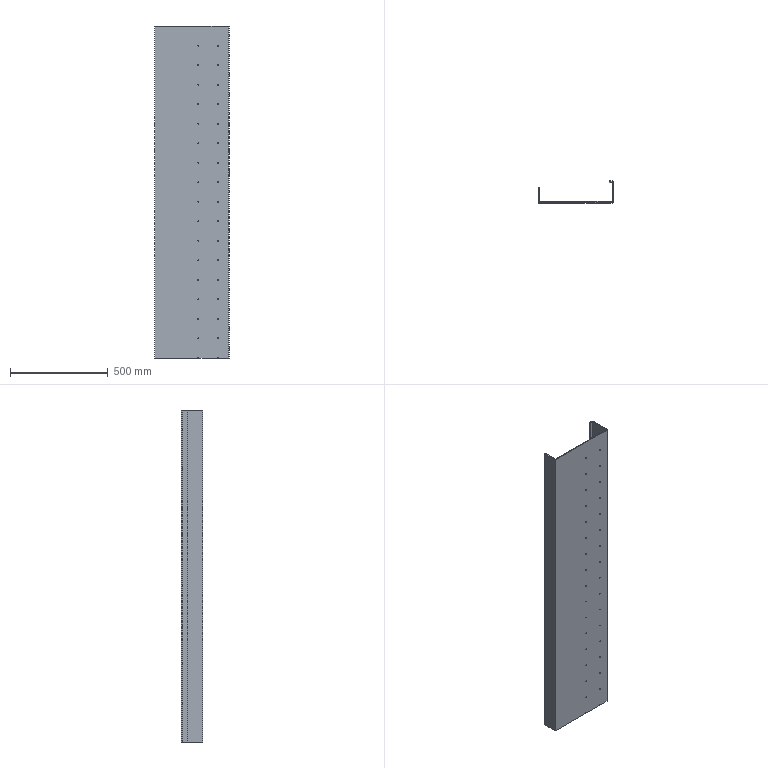Part | STEP file | Roller sheet metal_Mirror Default | 1 solid | 139 faces | box 380 x 110 x 1700 mm | volume 4838420 mm3 | cylinder 124 | plane 15 | commonest cylinder face diameters 5 x68 9 x34 6.8 x18 1 x2 11 x2